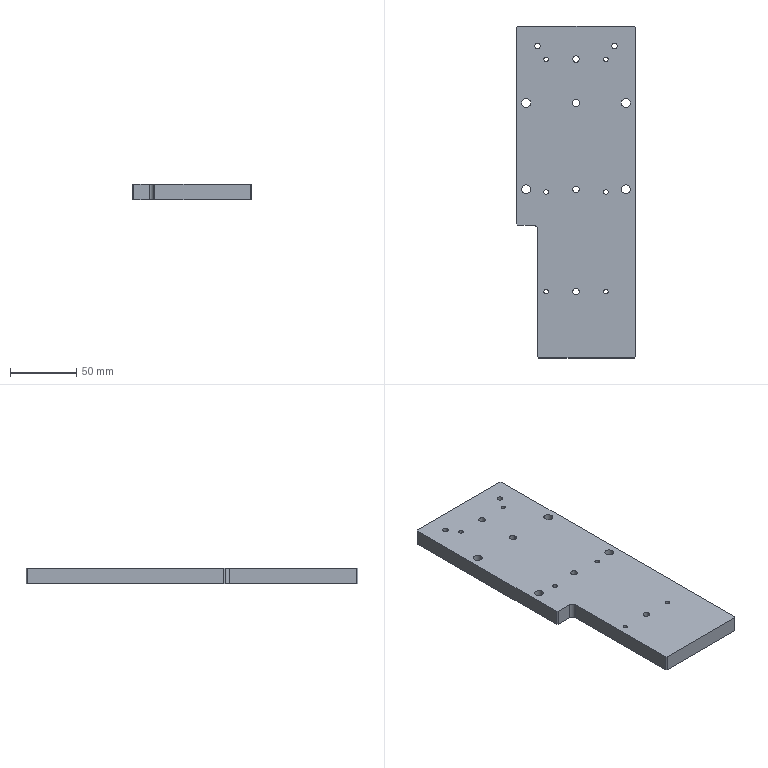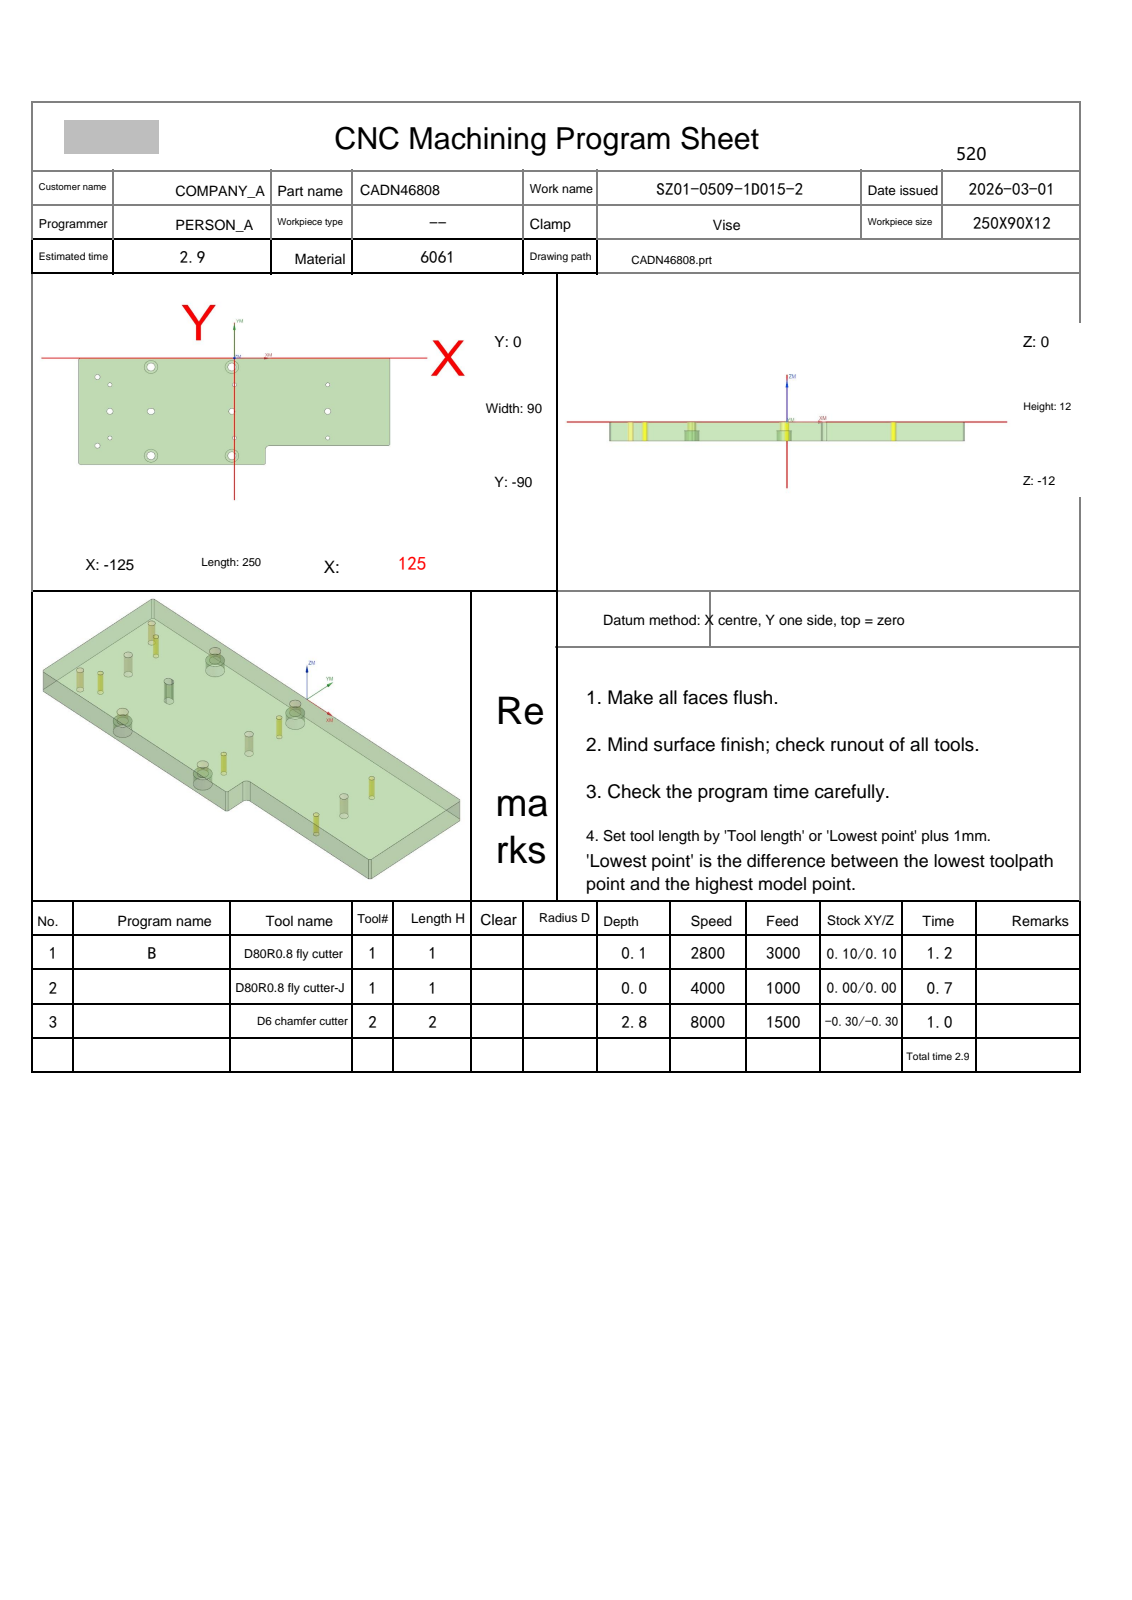NC program | NX | posted by the shop | part box 90 x 250 x 12 mm
Whole program:
%
O0001
(Machine time: 3.48 MIN)
(===Total Tool:2===)
(T1=D80R0.8 fly cutter D=80.  R=0.8  D-  H01 Z=0.    )
(T2=D6 chamfer cutter   D=6.   R=0.   D-  H02 Z=-2.8  )
G80 G90 G17 G49 G40
G91 G28 Z0
M01
N1 T01 M06
(D80R0.8 fly cutter  D=80. R=0.8 H=01 ce=0.10 di=0.10)
G00 G90 G54 X177.097 Y-66.097 M03 S2800
G43 H01 Z50.
M08
Z4.02
G01 Z2.02 F3000.
X165.097
X-157.897
G02 X-165.097 Y-58.897 I0.0 J7.2
G01 Y-39.263
G02 X-157.097 Y-31.263 I8. J0.0
G01 X165.097
X177.097
Z4.02
G00 Y-66.097
Z3.54
G01 Z1.54
X165.097
X-157.897
G02 X-165.097 Y-58.897 I0.0 J7.2
G01 Y-39.263
G02 X-157.097 Y-31.263 I8. J0.0
G01 X165.097
X177.097
Z3.54
G00 Y-66.097
Z3.06
G01 Z1.06
X165.097
X-157.897
G02 X-165.097 Y-58.897 I0.0 J7.2
G01 Y-39.263
G02 X-157.097 Y-31.263 I8. J0.0
G01 X165.097
X177.097
Z3.06
G00 Y-66.097
Z2.58
G01 Z.58
X165.097
X-157.897
G02 X-165.097 Y-58.897 I0.0 J7.2
G01 Y-39.263
G02 X-157.097 Y-31.263 I8. J0.0
G01 X165.097
X177.097
Z2.58
G00 Y-66.097
Z2.1
G01 Z.1
X165.097
X-157.897
G02 X-165.097 Y-58.897 I0.0 J7.2
G01 Y-39.263
G02 X-157.097 Y-31.263 I8. J0.0
G01 X165.097
X177.097
Z2.1
G00 Z50.
G91 G28 Z0.0
M05
M09
G91 G28 Z0.0
M01
N2 T01 M06
(D80R0.8 fly cutter-J  D=80. R=0.8 H=01 ce=0.00 di=0.00)
G00 G90 G54 X176.999 Y-65.999 M03 S4000
G43 H01 Z50.
M08
Z2.
G01 Z0.0 F1000.
X164.999
X-157.799
G02 X-164.999 Y-58.799 I0.0 J7.2
G01 Y-39.361
G02 X-156.999 Y-31.361 I8. J0.0
G01 X164.999
X176.999
Z2.
G00 Z50.
G91 G28 Z0.0
M05
M09
G91 G28 Z0.0
M01
N3 T02 M06
(D6 chamfer cutter  D=6. R=0. H=02 ce=0.00 di=0.00)
G00 G90 G54 X-100. Y-67.5 M03 S8000
G43 H02 Z50.
M08
G98 G81 X-100. Y-67.5 Z-2.2 R3. F1000.
Y-22.5
X0.0
Y-67.5
X75.
Y-22.5
G80
G00 Z50.
G00 G90 X-110. Y-74. M03 S8000
Z50.
G98 G81 X-110. Y-74. Z-2.7 R3. F1000.
Y-16.
G80
G00 Z50.
G00 G90 X75. Y-45. M03 S8000
Z50.
G98 G81 X75. Y-45. Z-2.8 R3. F1000.
X-2.
X-100.
G80
G00 Z50.
G00 G90 X-.913 Y-6.993 M03 S8000
Z50.
Z-.9
G01 Z-1.4 F1200.
X-.5 Y-6.8
G03 X-2. Y-5.3 I-1.5 J0.0
X-4.2 Y-7.5 I0.0 J-2.2
X-2. Y-9.7 I2.2 J0.0
X.2 Y-7.5 I0.0 J2.2
X-2. Y-5.3 I-2.2 J0.0
X-3.5 Y-6.8 I0.0 J-1.5
G01 X-3.087 Y-6.993
Z-.9
G00 Z50.
X-65.913
Z-.9
G01 Z-1.4
X-65.5 Y-6.8
G03 X-67. Y-5.3 I-1.5 J0.0
X-69.2 Y-7.5 I0.0 J-2.2
X-67. Y-9.7 I2.2 J0.0
X-64.8 Y-7.5 I0.0 J2.2
X-67. Y-5.3 I-2.2 J0.0
X-68.5 Y-6.8 I0.0 J-1.5
G01 X-68.087 Y-6.993
Z-.9
G00 Z50.
X-65.913 Y-81.993
Z-.9
G01 Z-1.4
X-65.5 Y-81.8
G03 X-67. Y-80.3 I-1.5 J0.0
X-69.2 Y-82.5 I0.0 J-2.2
X-67. Y-84.7 I2.2 J0.0
X-64.8 Y-82.5 I0.0 J2.2
X-67. Y-80.3 I-2.2 J0.0
X-68.5 Y-81.8 I0.0 J-1.5
G01 X-68.087 Y-81.993
Z-.9
G00 Z50.
X-.913
Z-.9
G01 Z-1.4
X-.5 Y-81.8
G03 X-2. Y-80.3 I-1.5 J0.0
X-4.2 Y-82.5 I0.0 J-2.2
X-2. Y-84.7 I2.2 J0.0
X.2 Y-82.5 I0.0 J2.2
X-2. Y-80.3 I-2.2 J0.0
X-3.5 Y-81.8 I0.0 J-1.5
G01 X-3.087 Y-81.993
Z-.9
G00 Z50.
G00 G90 X-.386 Y1.227 M03 S6500
Z50.
Z.172
G01 Z-1.2 F1500.
G03 X-.1 Y1.027 I1.286 J1.532
G01 X-.054 Y.997
X0.0 Y1.
X124.
X124.259 Y.966
X124.5 Y.866
X124.707 Y.707
X125.707 Y-.293
X125.866 Y-.5
X125.966 Y-.741
X126. Y-1.
Y-73.
X125.966 Y-73.259
X125.866 Y-73.5
X125.707 Y-73.707
X124.707 Y-74.707
X124.5 Y-74.866
X124.259 Y-74.966
X124. Y-75.
X28.
G03 X26. Y-77. I0.0 J-2.
G01 Y-89.
X25.966 Y-89.259
X25.866 Y-89.5
X25.707 Y-89.707
X24.707 Y-90.707
X24.5 Y-90.866
X24.259 Y-90.966
X24. Y-91.
X-124.
X-124.259 Y-90.966
X-124.5 Y-90.866
X-124.707 Y-90.707
X-125.707 Y-89.707
X-125.866 Y-89.5
X-125.966 Y-89.259
X-126. Y-89.
Y-1.
X-125.966 Y-.741
X-125.866 Y-.5
X-125.707 Y-.293
X-124.707 Y.707
X-124.5 Y.866
X-124.259 Y.966
X-124. Y1.
X0.0
X.054 Y.997
X.1 Y1.027
G03 X.386 Y1.227 I-1. J1.732
G01 Z.172
G00 Z10.
X75.419 Y-67.006
Z.405
G01 Z-1.2
G03 X75.103 Y-66.859 I-1. J-1.732
G01 X75.053 Y-66.838
X75. Y-66.85
G03 X74.35 Y-67.5 I0.0 J-.65
X75. Y-68.15 I.65 J0.0
X75.65 Y-67.5 I0.0 J.65
X75. Y-66.85 I-.65 J0.0
G01 X74.947 Y-66.838
X74.897 Y-66.859
G03 X74.581 Y-67.006 I.684 J-1.879
G01 Z.405
G00 Z10.
X75.407 Y-43.685
Z.284
G01 Z-1.2
G03 X75.102 Y-43.516 I-1.118 J-1.658
G01 X75.054 Y-43.491
X75. Y-43.5
G03 X73.5 Y-45. I0.0 J-1.5
X75. Y-46.5 I1.5 J0.0
X76.5 Y-45. I0.0 J1.5
X75. Y-43.5 I-1.5 J0.0
G01 X74.946 Y-43.491
X74.898 Y-43.516
G03 X74.593 Y-43.685 I.813 J-1.827
G01 Z.284
G00 Z10.
X75.419 Y-22.006
Z.405
G01 Z-1.2
G03 X75.103 Y-21.859 I-1. J-1.732
G01 X75.053 Y-21.838
X75. Y-21.85
G03 X74.35 Y-22.5 I0.0 J-.65
X75. Y-23.15 I.65 J0.0
X75.65 Y-22.5 I0.0 J.65
X75. Y-21.85 I-.65 J0.0
G01 X74.947 Y-21.838
X74.897 Y-21.859
G03 X74.581 Y-22.006 I.684 J-1.879
G01 Z.405
G00 Z10.
X-1.596 Y-5.392
Z.253
G01 Z-1.2
G03 X-1.898 Y-5.218 I-1.147 J-1.638
G01 X-1.946 Y-5.192
X-2. Y-5.2
G03 X-4.3 Y-7.5 I0.0 J-2.3
X-2. Y-9.8 I2.3 J0.0
X.3 Y-7.5 I0.0 J2.3
X-2. Y-5.2 I-2.3 J0.0
G01 X-2.054 Y-5.192
X-2.102 Y-5.218
G03 X-2.404 Y-5.392 I.845 J-1.813
G01 Z.253
G00 Z10.
X.419 Y-22.006
Z.405
G01 Z-1.2
G03 X.103 Y-21.859 I-1. J-1.732
G01 X.053 Y-21.838
X0.0 Y-21.85
G03 X-.65 Y-22.5 I0.0 J-.65
X0.0 Y-23.15 I.65 J0.0
X.65 Y-22.5 I0.0 J.65
X0.0 Y-21.85 I-.65 J0.0
G01 X-.053 Y-21.838
X-.103 Y-21.859
G03 X-.419 Y-22.006 I.684 J-1.879
G01 Z.405
G00 Z10.
X-1.593 Y-43.685
Z.284
G01 Z-1.2
G03 X-1.898 Y-43.516 I-1.118 J-1.658
G01 X-1.946 Y-43.491
X-2. Y-43.5
G03 X-3.5 Y-45. I0.0 J-1.5
X-2. Y-46.5 I1.5 J0.0
X-.5 Y-45. I0.0 J1.5
X-2. Y-43.5 I-1.5 J0.0
G01 X-2.054 Y-43.491
X-2.102 Y-43.516
G03 X-2.407 Y-43.685 I.813 J-1.827
G01 Z.284
G00 Z10.
X.419 Y-67.006
Z.405
G01 Z-1.2
G03 X.103 Y-66.859 I-1. J-1.732
G01 X.053 Y-66.838
X0.0 Y-66.85
G03 X-.65 Y-67.5 I0.0 J-.65
X0.0 Y-68.15 I.65 J0.0
X.65 Y-67.5 I0.0 J.65
X0.0 Y-66.85 I-.65 J0.0
G01 X-.053 Y-66.838
X-.103 Y-66.859
G03 X-.419 Y-67.006 I.684 J-1.879
G01 Z.405
G00 Z10.
X-1.596 Y-80.392
Z.253
G01 Z-1.2
G03 X-1.898 Y-80.218 I-1.147 J-1.638
G01 X-1.946 Y-80.192
X-2. Y-80.2
G03 X-4.3 Y-82.5 I0.0 J-2.3
X-2. Y-84.8 I2.3 J0.0
X.3 Y-82.5 I0.0 J2.3
X-2. Y-80.2 I-2.3 J0.0
G01 X-2.054 Y-80.192
X-2.102 Y-80.218
G03 X-2.404 Y-80.392 I.845 J-1.813
G01 Z.253
G00 Z10.
X-66.596
Z.253
G01 Z-1.2
G03 X-66.898 Y-80.218 I-1.147 J-1.638
G01 X-66.946 Y-80.192
X-67. Y-80.2
G03 X-69.3 Y-82.5 I0.0 J-2.3
X-67. Y-84.8 I2.3 J0.0
X-64.7 Y-82.5 I0.0 J2.3
X-67. Y-80.2 I-2.3 J0.0
G01 X-67.054 Y-80.192
X-67.102 Y-80.218
G03 X-67.404 Y-80.392 I.845 J-1.813
G01 Z.253
G00 Z10.
X-67.386 Y-46.273
Z.172
G01 Z-1.2
G03 X-67.1 Y-46.473 I1.286 J1.532
G01 X-67.054 Y-46.503
X-67. Y-46.5
X-66.5
G03 X-65. Y-45. I0.0 J1.5
X-66.5 Y-43.5 I-1.5 J0.0
G01 X-67.5
G03 X-69. Y-45. I0.0 J-1.5
X-67.5 Y-46.5 I1.5 J0.0
G01 X-67.
X-66.946 Y-46.503
X-66.9 Y-46.473
G03 X-66.614 Y-46.273 I-1. J1.732
G01 Z.172
G00 Z10.
X-66.596 Y-5.392
Z.253
G01 Z-1.2
G03 X-66.898 Y-5.218 I-1.147 J-1.638
G01 X-66.946 Y-5.192
X-67. Y-5.2
G03 X-69.3 Y-7.5 I0.0 J-2.3
X-67. Y-9.8 I2.3 J0.0
X-64.7 Y-7.5 I0.0 J2.3
X-67. Y-5.2 I-2.3 J0.0
G01 X-67.054 Y-5.192
X-67.102 Y-5.218
G03 X-67.404 Y-5.392 I.845 J-1.813
G01 Z.253
G00 Z10.
X-110.412 Y-16.926
Z.32
G01 Z-1.2
G03 X-110.103 Y-17.086 I1.075 J1.687
G01 X-110.054 Y-17.11
X-110. Y-17.1
G03 X-108.9 Y-16. I0.0 J1.1
X-110. Y-14.9 I-1.1 J0.0
X-111.1 Y-16. I0.0 J-1.1
X-110. Y-17.1 I1.1 J0.0
G01 X-109.946 Y-17.11
X-109.897 Y-17.086
G03 X-109.588 Y-16.926 I-.765 J1.848
G01 Z.32
G00 Z2.55
X-99.581 Y-22.006
Z.405
G01 Z-1.2
G03 X-99.897 Y-21.859 I-1. J-1.732
G01 X-99.947 Y-21.838
X-100. Y-21.85
G03 X-100.65 Y-22.5 I0.0 J-.65
X-100. Y-23.15 I.65 J0.0
X-99.35 Y-22.5 I0.0 J.65
X-100. Y-21.85 I-.65 J0.0
G01 X-100.053 Y-21.838
X-100.103 Y-21.859
G03 X-100.419 Y-22.006 I.684 J-1.879
G01 Z.405
G00 Z10.
X-99.593 Y-43.685
Z.284
G01 Z-1.2
G03 X-99.898 Y-43.516 I-1.118 J-1.658
G01 X-99.946 Y-43.491
X-100. Y-43.5
G03 X-101.5 Y-45. I0.0 J-1.5
X-100. Y-46.5 I1.5 J0.0
X-98.5 Y-45. I0.0 J1.5
X-100. Y-43.5 I-1.5 J0.0
G01 X-100.054 Y-43.491
X-100.102 Y-43.516
G03 X-100.407 Y-43.685 I.813 J-1.827
G01 Z.284
G00 Z10.
X-99.581 Y-67.006
Z.405
G01 Z-1.2
G03 X-99.897 Y-66.859 I-1. J-1.732
G01 X-99.947 Y-66.838
X-100. Y-66.85
G03 X-100.65 Y-67.5 I0.0 J-.65
X-100. Y-68.15 I.65 J0.0
X-99.35 Y-67.5 I0.0 J.65
X-100. Y-66.85 I-.65 J0.0
G01 X-100.053 Y-66.838
X-100.103 Y-66.859
G03 X-100.419 Y-67.006 I.684 J-1.879
G01 Z.405
G00 Z10.
X-110.412 Y-74.926
Z.32
G01 Z-1.2
G03 X-110.103 Y-75.086 I1.075 J1.687
G01 X-110.054 Y-75.11
X-110. Y-75.1
G03 X-108.9 Y-74. I0.0 J1.1
X-110. Y-72.9 I-1.1 J0.0
X-111.1 Y-74. I0.0 J-1.1
X-110. Y-75.1 I1.1 J0.0
G01 X-109.946 Y-75.11
X-109.897 Y-75.086
G03 X-109.588 Y-74.926 I-.765 J1.848
G01 Z.32
G00 Z50.
M05
M09
G91 G28 Z0.0
G91 G28 Y0.0
M30
%